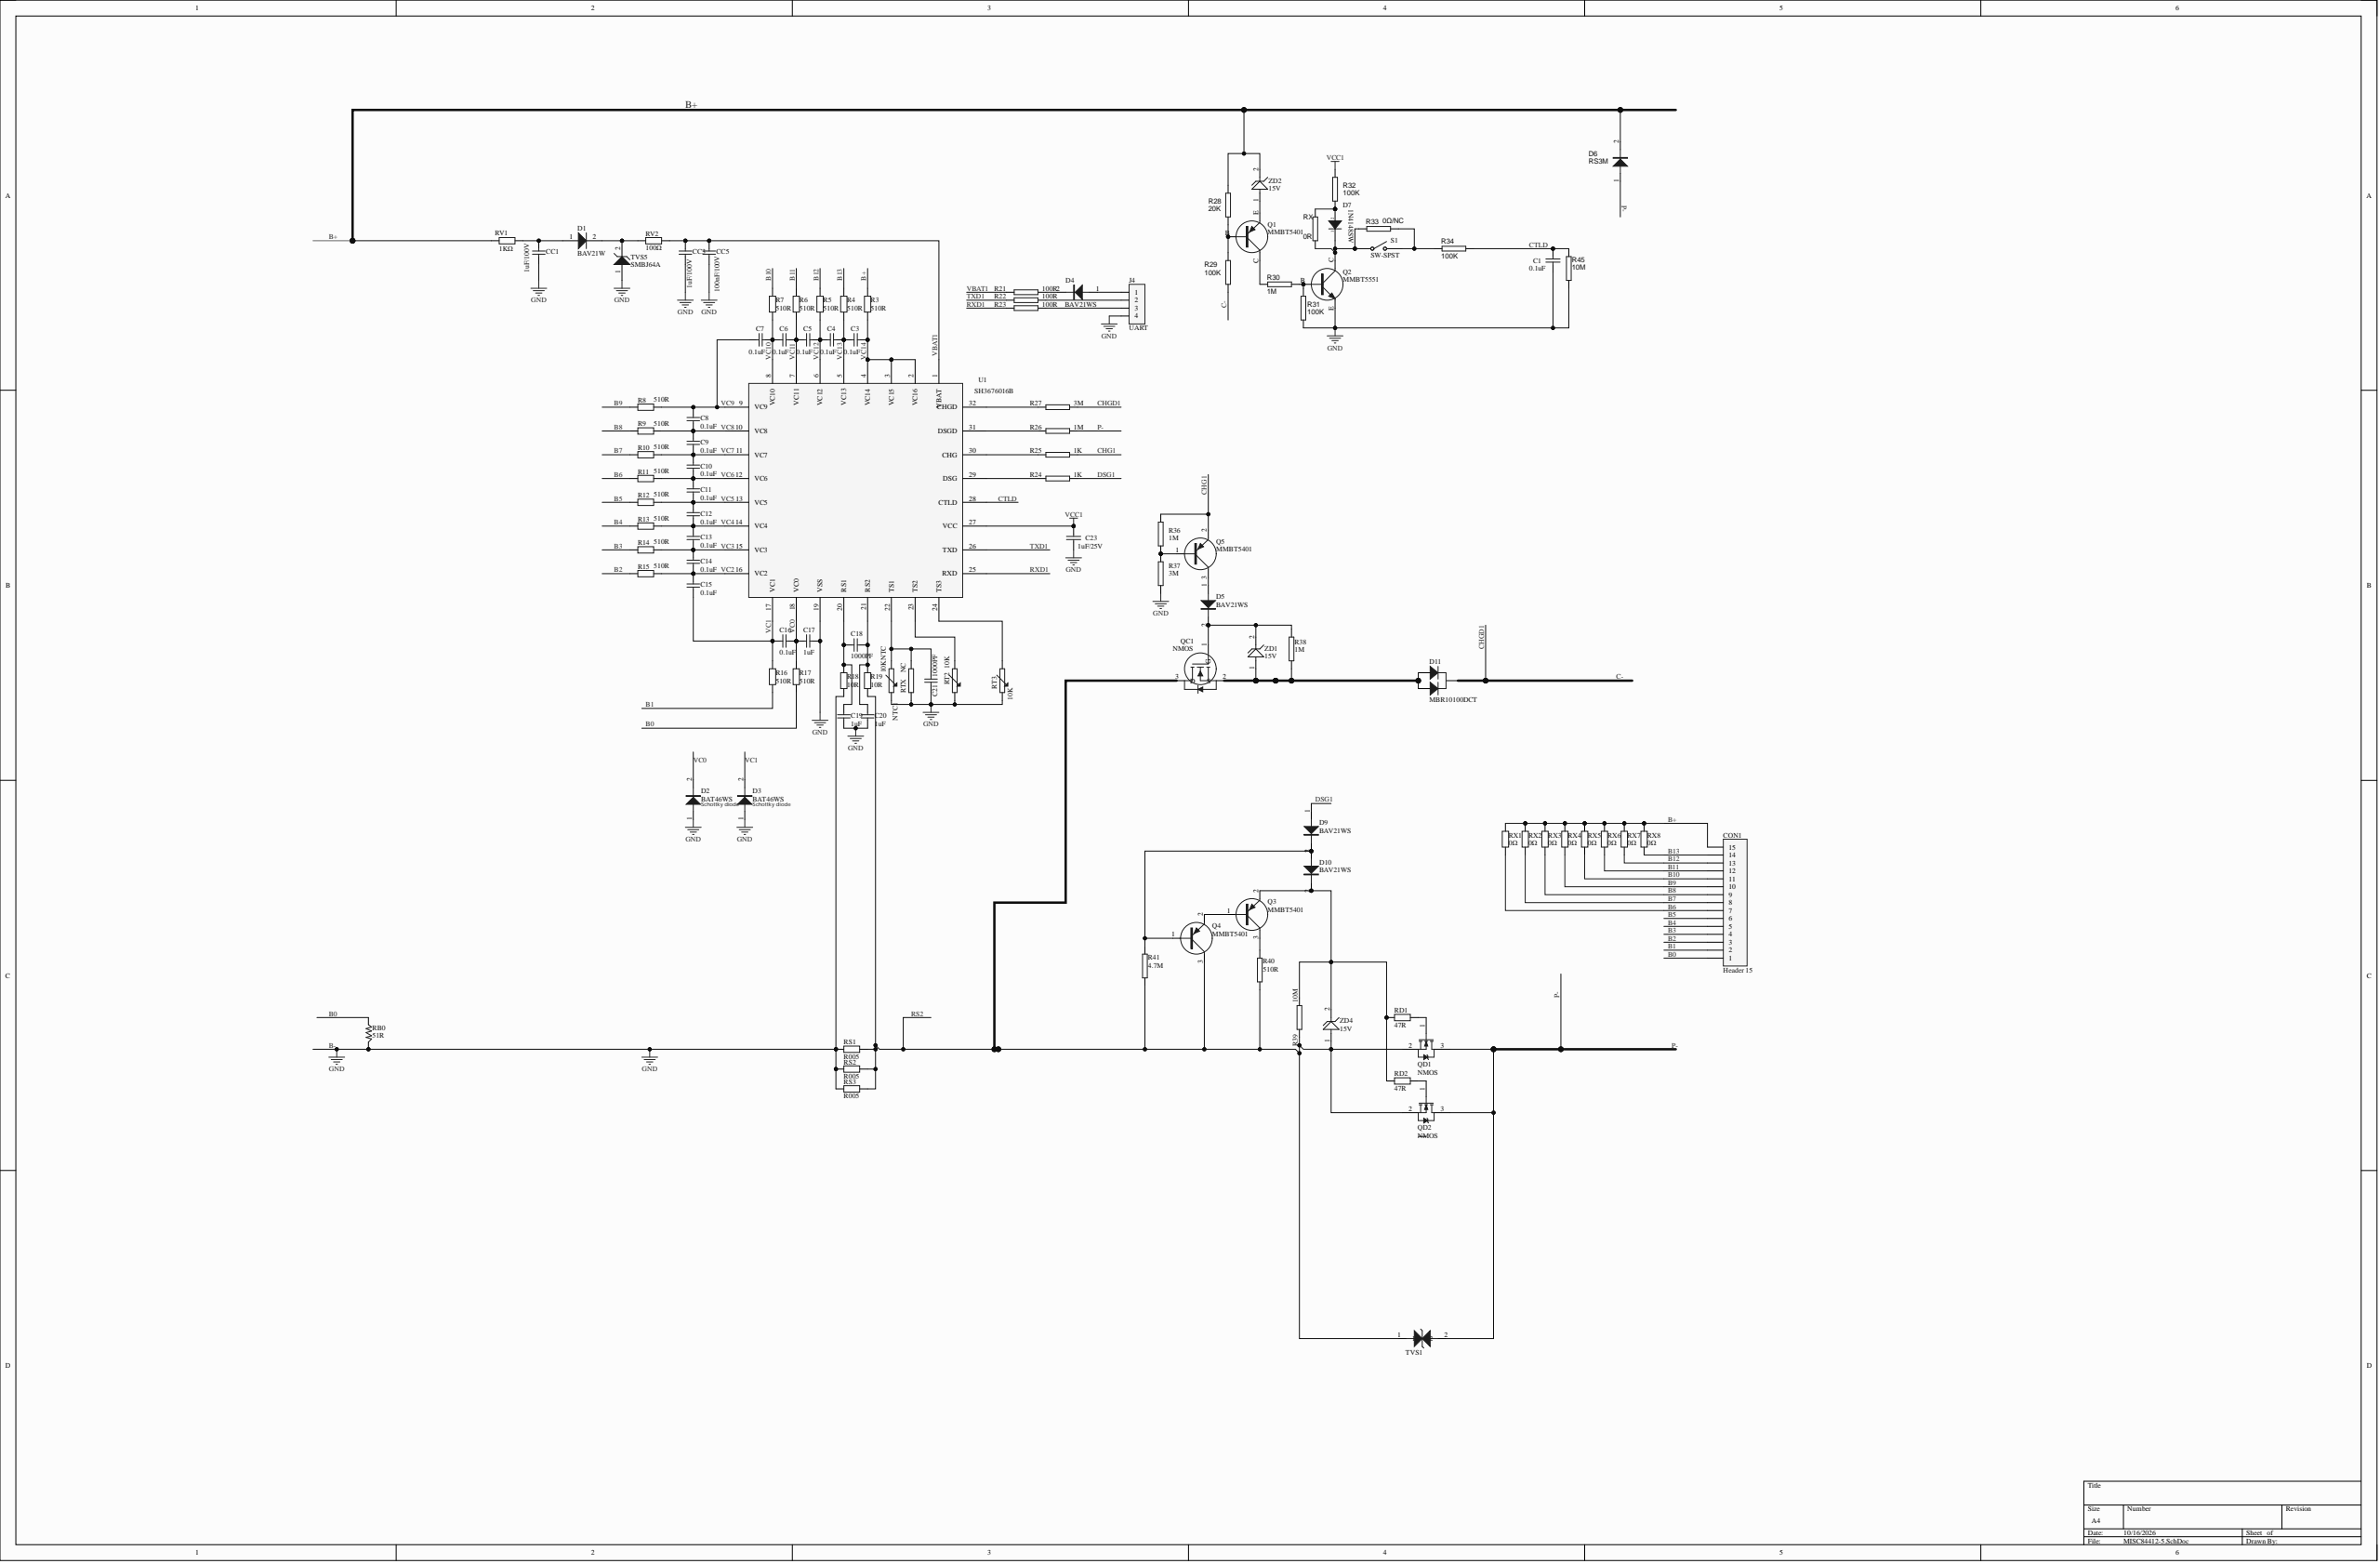Circuit board | Altium Designer | 110 parts | 73 nets
Bill of materials:
Comment,Description,Designator,Footprint,LibRef,Quantity
"0.1uF","CAP","C1","C0603A","CAP","1"
"0.1uF","SMD capacitor","C3, C4, C5, C6, C7, C8, C9, C10, C11, C12, C13, C14, C15, C16","C0402A","0805 100nF(104) 10% 50V","14"
"1uF","SMD capacitor","C17, C19, C20","C0402A","0805 100nF(104) 10% 50V","3"
"1000PF","SMD capacitor","C18","C0402A","0805 100nF(104) 10% 50V","1"
"1000PF","SMD capacitor","C21","C0603A","0805 100nF(104) 10% 50V","1"
"1uF/25V","CAP","C23","C0603A","CAP","1"
"1uF/100V","SMD capacitor","CC1, CC3","C0805L","0805 100nF(104) 10% 50V","2"
"100nF/100V","SMD capacitor","CC5","C0603A","0805 100nF(104) 10% 50V","1"
"Header 15","Header15","CON1","PH-2.0mm15P弯脚不带扣","Header 15","1"
"BAV21W","Diode","D1","SOD323(1+2-)","SOD-323 1N4148WS T4","1"
"BAT46WS","DIODE","D2, D3","SOD323(1+2-)","DIODE","2"
"BAV21WS","DIODE","D4, D5, D9, D10","SOD323(1+2-)","DIODE","4"
"RS3M","DIODE","D6","SMB M(1+2-)","DIODE","1"
"1N4148SW","SMD diode","D7","SOD323","1N4148SW","1"
"MBR10100DCT","SMD dual diode, common cathode","D11","TO-252-DIODE-DUAL","MBR10100DCT","1"
"UART","","J4","CH-2.0-4P","CON4","1"
"10KNTC","RES","NTC1","RT2.3X1-2","RES2","1"
"MMBT5401","PNP Transistor","Q1","SOT23-3_BEC","PNP","1"
"MMBT5551","NPN Transistor","Q2","SOT23-3_BEC","NPN","1"
"MMBT5401","PNP","Q3, Q4, Q5","SOT23-3","8550","3"
"NMOS","","QC1","TO-252-DFN","MOSFET-N","1"
"NMOS","HEXFET N-Channel Power MOSFET","QD1, QD2","TOLL","IRFR014","2"
"510R","SMD resistor","R3, R4, R5, R6, R7, R8, R9, R10, R11, R12, R13, R14, R15, R16, R17","R0402A","0603 1KΩ (1001) 1%","15"
"10R","SMD resistor","R18, R19","R0402A","0603 1KΩ (1001) 1%","2"
"100R","RES","R21, R22, R23","R0402A","RES1","3"
"1K","RES","R24, R25","R0603A","RES1","2"
"1M","RES","R26, R30, R36, R38","R0603A","RES1","4"
"3M","RES","R27, R37","R0603A","RES1","2"
"20K","RES","R28","R0603A","RES1","1"
"100K","RES","R29, R31, R32, R34","R0603A","RES1","4"
"0Ω/NC","RES","R33","R0603A","RES1","1"
"10M","RES","R39","R0402A","RES1","1"
"510R","RES","R40","R0603A","RES1","1"
"4.7M","RES","R41","R0603A","RES1","1"
"10M","RES","R45","R0603A","RES1","1"
"51R","±5% /UniOhm/yageo/TA-I/Walsin/Ralec","RB0","R0805L","RES1","1"
"47R","SMD resistor","RD1, RD2","R0603Ap","0603 1.2MΩ (1204) 1%","2"
"R005","SMD resistor","RS1, RS2, RS3","R2512L","0603 1KΩ (1001) 1%","3"
"10K","RES","RT2, RT3","R0603A","RES2","2"
"NC","RES","RTX","R0603A","RES1","1"
"1KΩ","SMD resistor","RV1","R0805L","0805 300Ω (3000) 1%","1"
"100Ω","SMD resistor","RV2","R0805L","0805 300Ω (3000) 1%","1"
"0R","RES","RX","R0603A","RES1","1"
"0Ω","SMD resistor","RX1, RX2, RX3, RX4, RX5, RX6, RX7, RX8","R0805L","0805 300Ω (3000) 1%","8"
"SW-SPST","Single-Pole, Single-Throw Switch","S1","RT2.3X1.2-2","SW-SPST","1"
"75CA","TVS","TVS1","SMC_M(DO-214AB)","TVS","1"
"SMBJ64A","Zener diode","TVS5","SMB M(1+2-)","LL-34 ZMM5V6","1"
"SH3676016B","SH3676016B","U1","LQFP32L(PIN间距0.8mm)","SH3676016B","1"
"15V","ZENOR","ZD1, ZD2, ZD4","SOD323(1+2-)","ZENOR","3"
Netlist (Protel format):
[
C1
C0603A
0.1uF



]
[
C3
C0402A
0.1uF



]
[
C4
C0402A
0.1uF



]
[
C5
C0402A
0.1uF



]
[
C6
C0402A
0.1uF



]
[
C7
C0402A
0.1uF



]
[
C8
C0402A
0.1uF



]
[
C9
C0402A
0.1uF



]
[
C10
C0402A
0.1uF



]
[
C11
C0402A
0.1uF



]
[
C12
C0402A
0.1uF



]
[
C13
C0402A
0.1uF



]
[
C14
C0402A
0.1uF



]
[
C15
C0402A
0.1uF



]
[
C16
C0402A
0.1uF



]
[
C17
C0402A
1uF



]
[
C18
C0402A
1000PF



]
[
C19
C0402A
1uF



]
[
C20
C0402A
1uF



]
[
C21
C0603A
1000PF



]
[
C23
C0603A
1uF/25V



]
[
CC1
C0805L
1uF/100V



]
[
CC3
C0805L
1uF/100V



]
[
CC5
C0603A
100nF/100V



]
[
CON1
PH-2.0mm15P弯脚不带扣
Header 15



]
[
D1
SOD323(1+2-)
BAV21W



]
[
D2
SOD323(1+2-)
BAT46WS



]
[
D3
SOD323(1+2-)
BAT46WS



]
[
D4
SOD323(1+2-)
BAV21WS



]
[
D5
SOD323(1+2-)
BAV21WS



]
[
D6
SMB M(1+2-)
RS3M



]
[
D7
SOD323
1N4148SW



]
[
D9
SOD323(1+2-)
BAV21WS



]
[
D10
SOD323(1+2-)
BAV21WS



]
[
D11
TO-252-DIODE-DUAL
MBR10100DCT



]
[
J4
CH-2.0-4P
UART



]
[
NTC1
RT2.3X1-2
10KNTC



]
[
Q1
SOT23-3_BEC
MMBT5401



]
[
Q2
SOT23-3_BEC
MMBT5551



]
[
Q3
SOT23-3
MMBT5401



]
[
Q4
SOT23-3
MMBT5401



]
[
Q5
SOT23-3
MMBT5401



]
[
QC1
TO-252-DFN
NMOS



]
[
QD1
TOLL
NMOS



]
[
QD2
TOLL
NMOS



]
[
R3
R0402A
510R



]
[
R4
R0402A
510R



]
[
R5
R0402A
510R



]
[
R6
R0402A
510R



]
[
R7
R0402A
510R



]
[
R8
R0402A
510R



]
[
R9
R0402A
510R



]
[
R10
R0402A
510R



]
[
R11
R0402A
510R



]
[
R12
R0402A
510R



]
[
R13
R0402A
510R



]
[
R14
R0402A
510R



]
[
R15
R0402A
510R



]
[
R16
R0402A
510R



]
[
R17
R0402A
510R



]
[
R18
R0402A
10R



]
[
R19
R0402A
10R



]
[
R21
R0402A
100R



]
[
R22
R0402A
100R



]
[
R23
R0402A
100R



]
[
R24
R0603A
1K



]
[
R25
R0603A
1K



]
[
R26
R0603A
1M



]
[
R27
R0603A
3M



]
[
R28
R0603A
20K



]
[
R29
R0603A
100K



]
[
R30
R0603A
1M



]
[
R31
R0603A
100K



]
[
R32
R0603A
100K



]
[
R33
R0603A
0Ω/NC



]
[
R34
R0603A
100K



]
[
R36
R0603A
1M



]
[
R37
R0603A
3M



]
[
R38
R0603A
1M



]
[
R39
R0402A
10M



]
[
R40
R0603A
510R



]
[
R41
R0603A
4.7M



]
[
R45
R0603A
10M



]
[
RB0
R0805L
51R



]
[
RD1
R0603Ap
47R



]
[
RD2
R0603Ap
47R



]
[
RS1
R2512L
R005



]
[
RS2
R2512L
R005



]
[
RS3
R2512L
R005



]
[
RT2
R0603A
10K



]
[
RT3
R0603A
10K



]
[
RTX
R0603A
NC



]
[
RV1
R0805L
1KΩ



]
[
RV2
R0805L
100Ω



]
[
RX
R0603A
0R



]
[
RX1
R0805L
0Ω



]
[
RX2
R0805L
0Ω



]
[
RX3
R0805L
0Ω



]
[
RX4
R0805L
0Ω



]
[
RX5
R0805L
0Ω



]
[
RX6
R0805L
0Ω



]
[
RX7
R0805L
0Ω



]
[
RX8
R0805L
0Ω



]
[
S1
RT2.3X1.2-2
SW-SPST



]
[
TVS1
SMC_M(DO-214AB)
75CA



]
[
TVS5
SMB M(1+2-)
SMBJ64A



]
[
U1
LQFP32L(PIN间距0.8mm)
SH3676016B



]
[
ZD1
SOD323(1+2-)
15V



]
[
ZD2
SOD323(1+2-)
15V



]
[
ZD4
SOD323(1+2-)
15V



]
(
VCC1
C23-2
R32-1
U1-27
)
(
VC14
C3-2
R3-1
U1-2
U1-3
U1-4
)
(
VC13
C3-1
C4-2
R4-1
U1-5
)
(
VC12
C4-1
C5-2
R5-1
U1-6
)
(
VC11
C5-1
C6-2
R6-1
U1-7
)
(
VC10
C6-1
C7-2
R7-1
U1-8
)
(
VC9
C7-1
C8-2
R8-1
U1-9
)
(
VC8
C8-1
C9-2
R9-1
U1-10
)
(
VC7
C9-1
C10-2
R10-1
U1-11
)
(
VC6
C10-1
C11-2
R11-1
U1-12
)
(
VC5
C11-1
C12-2
R12-1
U1-13
)
(
VC4
C12-1
C13-2
R13-1
U1-14
)
(
VC3
C13-1
C14-2
R14-1
U1-15
)
(
VC2
C14-1
C15-2
R15-2
U1-16
)
(
VC1
C15-1
C16-2
D3-2
R16-1
U1-17
)
(
VC0
C16-1
C17-2
D2-2
R17-1
U1-18
)
(
VBAT1
CC3-2
CC5-2
R21-2
RV2-1
U1-1
)
(
TXD1
R22-2
U1-26
)
(
RXD1
R23-2
U1-25
)
(
RS2
Q4-3
QC1-3
QD1-2
QD2-2
R19-2
R39-1
R40-2
R41-1
RS1-2
RS2-2
RS3-2
TVS1-1
ZD4-1
)
(
P-
D6-1
QD1-3
QD2-3
R26-1
TVS1-2
)
(
NetRT3_1
RT3-1
U1-24
)
(
NetRT2_1
RT2-1
U1-23
)
(
NetR33_1
R33-1
R34-1
S1-2
)
(
NetR27_2
R27-2
U1-32
)
(
NetR26_2
R26-2
U1-31
)
(
NetR25_2
R25-2
U1-30
)
(
NetR24_2
R24-2
U1-29
)
(
NetQD2_1
QD2-1
RD2-2
)
(
NetQD1_1
QD1-1
RD1-2
)
(
NetQ5_1
Q5-1
R36-1
R37-1
)
(
NetQ3_3
Q3-3
R40-1
)
(
NetQ3_1
Q3-1
Q4-2
)
(
NetQ2_B
Q2-B
R30-1
R31-2
)
(
NetQ1_E
Q1-E
ZD2-1
)
(
NetQ1_C
Q1-C
R30-2
)
(
NetQ1_B
Q1-B
R28-1
R29-2
)
(
NetJ4_3
J4-3
R23-1
)
(
NetJ4_2
J4-2
R22-1
)
(
NetD11_1
D11-1
D11-2
QC1-2
R38-1
ZD1-1
)
(
NetD10_2
D10-2
Q3-2
R39-2
RD1-1
RD2-1
ZD4-2
)
(
NetD9_2
D9-2
D10-1
Q4-1
R41-2
)
(
NetD7_2
D7-2
R32-2
RX-2
)
(
NetD7_1
D7-1
Q2-C
R33-2
RX-1
S1-1
)
(
NetD5_2
D5-2
QC1-1
R38-2
ZD1-2
)
(
NetD5_1
D5-1
Q5-3
)
(
NetD4_2
D4-2
R21-1
)
(
NetD4_1
D4-1
J4-1
)
(
NetD1_2
D1-2
RV2-2
TVS5-2
)
(
NetCC1_2
CC1-2
D1-1
RV1-1
)
(
NetC21_1
C21-1
NTC1-1
RTX-1
U1-22
)
(
NetC18_2
C18-2
C19-1
R18-1
U1-20
)
(
NetC18_1
C18-1
C20-1
R19-1
U1-21
)
(
DSG1
D9-1
R24-1
)
(
CTLD
C1-1
R34-2
R45-1
U1-28
)
(
CHG1
Q5-2
R25-1
R36-2
)
(
C-
D11-3
R27-1
R29-1
)
(
B-
C1-2
C17-1
C19-2
C20-2
C21-2
C23-1
CC1-1
CC3-1
CC5-1
D2-1
D3-1
J4-4
NTC1-2
Q2-E
R18-2
R31-1
R37-2
R45-2
RB0-1
RS1-1
RS2-1
RS3-1
RT2-2
RT3-2
RTX-2
TVS5-1
U1-19
)
(
B+
CON1-15
D6-2
R3-2
R28-2
RV1-2
RX1-1
RX2-1
RX3-1
RX4-1
RX5-1
RX6-1
RX7-1
RX8-1
ZD2-2
)
(
B13
CON1-14
R4-2
RX8-2
)
(
B12
CON1-13
R5-2
RX7-2
)
(
B11
CON1-12
R6-2
RX6-2
)
(
B10
CON1-11
R7-2
RX5-2
)
(
B9
CON1-10
R8-2
RX4-2
)
(
B8
CON1-9
R9-2
RX3-2
)
(
B7
CON1-8
R10-2
RX2-2
)
(
B6
CON1-7
R11-2
RX1-2
)
(
B5
CON1-6
R12-2
)
(
B4
CON1-5
R13-2
)
(
B3
CON1-4
R14-2
)
(
B2
CON1-3
R15-1
)
(
B1
CON1-2
R16-2
)
(
B0
CON1-1
R17-2
RB0-2
)